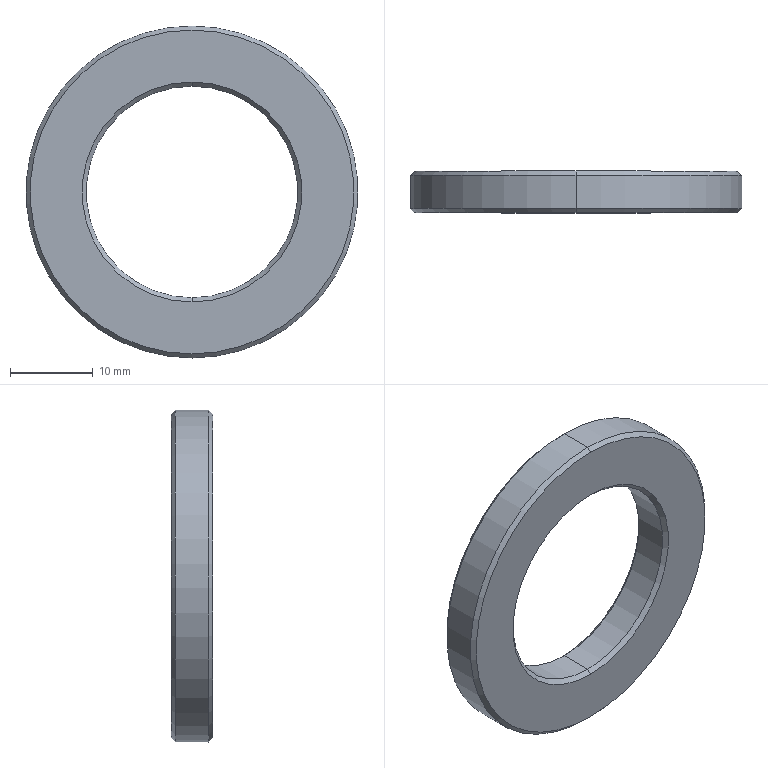Part | SolidWorks | features BaseBody 1 | 1 solid | 14 faces | box 40 x 5 x 40 mm | volume 3678 mm3 | cone 8 | cylinder 4 | plane 2 | commonest cylinder face diameters 25.5 x2 40 x2
STEP:
#1=CARTESIAN_POINT('',(0.,4.5,-12.75));
#2=VERTEX_POINT('',#1);
#3=CARTESIAN_POINT('',(0.,4.5,12.75));
#4=VERTEX_POINT('',#3);
#5=CARTESIAN_POINT('',(0.,4.5,0.));
#6=DIRECTION('',(0.,1.,0.));
#7=DIRECTION('',(0.,0.,-1.));
#8=AXIS2_PLACEMENT_3D('',#5,#6,#7);
#9=CIRCLE('',#8,12.75);
#10=EDGE_CURVE('',#2,#4,#9,.T.);
#11=ORIENTED_EDGE('',*,*,#10,.F.);
#12=CARTESIAN_POINT('',(0.,5.,-13.25));
#13=VERTEX_POINT('',#12);
#14=CARTESIAN_POINT('',(0.,5.,-13.25));
#15=DIRECTION('',(0.,0.7071,-0.7071));
#16=VECTOR('',#15,1000.);
#17=LINE('',#14,#16);
#18=EDGE_CURVE('',#2,#13,#17,.T.);
#19=ORIENTED_EDGE('',*,*,#18,.T.);
#20=CARTESIAN_POINT('',(0.,5.,13.25));
#21=VERTEX_POINT('',#20);
#22=CARTESIAN_POINT('',(0.,5.,0.));
#23=DIRECTION('',(0.,-1.,0.));
#24=DIRECTION('',(0.,0.,1.));
#25=AXIS2_PLACEMENT_3D('',#22,#23,#24);
#26=CIRCLE('',#25,13.25);
#27=EDGE_CURVE('',#21,#13,#26,.T.);
#28=ORIENTED_EDGE('',*,*,#27,.F.);
#29=CARTESIAN_POINT('',(0.,5.,13.25));
#30=DIRECTION('',(0.,0.7071,0.7071));
#31=VECTOR('',#30,1000.);
#32=LINE('',#29,#31);
#33=EDGE_CURVE('',#4,#21,#32,.T.);
#34=ORIENTED_EDGE('',*,*,#33,.F.);
#35=EDGE_LOOP('',(#11,#19,#28,#34));
#36=FACE_OUTER_BOUND('',#35,.T.);
#37=CARTESIAN_POINT('',(0.,5.,0.));
#38=DIRECTION('',(0.,1.,0.));
#39=DIRECTION('',(0.,0.,1.));
#40=AXIS2_PLACEMENT_3D('',#37,#38,#39);
#41=CONICAL_SURFACE('',#40,13.25,0.7854);
#42=ADVANCED_FACE('',(#36),#41,.F.);
#43=CARTESIAN_POINT('',(0.,5.,19.5));
#44=VERTEX_POINT('',#43);
#45=CARTESIAN_POINT('',(0.,5.,-19.5));
#46=VERTEX_POINT('',#45);
#47=CARTESIAN_POINT('',(0.,5.,0.));
#48=DIRECTION('',(0.,1.,0.));
#49=DIRECTION('',(0.,0.,-1.));
#50=AXIS2_PLACEMENT_3D('',#47,#48,#49);
#51=CIRCLE('',#50,19.5);
#52=EDGE_CURVE('',#44,#46,#51,.T.);
#53=ORIENTED_EDGE('',*,*,#52,.F.);
#54=CARTESIAN_POINT('',(0.,4.5,20.));
#55=VERTEX_POINT('',#54);
#56=CARTESIAN_POINT('',(0.,4.5,20.));
#57=DIRECTION('',(0.,-0.7071,0.7071));
#58=VECTOR('',#57,1000.);
#59=LINE('',#56,#58);
#60=EDGE_CURVE('',#44,#55,#59,.T.);
#61=ORIENTED_EDGE('',*,*,#60,.T.);
#62=CARTESIAN_POINT('',(0.,4.5,-20.));
#63=VERTEX_POINT('',#62);
#64=CARTESIAN_POINT('',(0.,4.5,0.));
#65=DIRECTION('',(0.,1.,0.));
#66=DIRECTION('',(0.,0.,-1.));
#67=AXIS2_PLACEMENT_3D('',#64,#65,#66);
#68=CIRCLE('',#67,20.);
#69=EDGE_CURVE('',#55,#63,#68,.T.);
#70=ORIENTED_EDGE('',*,*,#69,.T.);
#71=CARTESIAN_POINT('',(0.,4.5,-20.));
#72=DIRECTION('',(0.,-0.7071,-0.7071));
#73=VECTOR('',#72,1000.);
#74=LINE('',#71,#73);
#75=EDGE_CURVE('',#46,#63,#74,.T.);
#76=ORIENTED_EDGE('',*,*,#75,.F.);
#77=EDGE_LOOP('',(#53,#61,#70,#76));
#78=FACE_OUTER_BOUND('',#77,.T.);
#79=CARTESIAN_POINT('',(0.,4.5,0.));
#80=DIRECTION('',(0.,-1.,0.));
#81=DIRECTION('',(0.,0.,-1.));
#82=AXIS2_PLACEMENT_3D('',#79,#80,#81);
#83=CONICAL_SURFACE('',#82,20.,0.7854);
#84=ADVANCED_FACE('',(#78),#83,.T.);
#85=CARTESIAN_POINT('',(0.,0.5,-12.75));
#86=VERTEX_POINT('',#85);
#87=CARTESIAN_POINT('',(0.,0.5,12.75));
#88=VERTEX_POINT('',#87);
#89=CARTESIAN_POINT('',(0.,0.5,0.));
#90=DIRECTION('',(0.,1.,0.));
#91=DIRECTION('',(0.,0.,1.));
#92=AXIS2_PLACEMENT_3D('',#89,#90,#91);
#93=CIRCLE('',#92,12.75);
#94=EDGE_CURVE('',#86,#88,#93,.T.);
#95=ORIENTED_EDGE('',*,*,#94,.F.);
#96=CARTESIAN_POINT('',(0.,0.,-12.75));
#97=DIRECTION('',(0.,1.,0.));
#98=VECTOR('',#97,1000.);
#99=LINE('',#96,#98);
#100=EDGE_CURVE('',#86,#2,#99,.T.);
#101=ORIENTED_EDGE('',*,*,#100,.T.);
#102=ORIENTED_EDGE('',*,*,#10,.T.);
#103=CARTESIAN_POINT('',(0.,0.,12.75));
#104=DIRECTION('',(0.,1.,0.));
#105=VECTOR('',#104,1000.);
#106=LINE('',#103,#105);
#107=EDGE_CURVE('',#88,#4,#106,.T.);
#108=ORIENTED_EDGE('',*,*,#107,.F.);
#109=EDGE_LOOP('',(#95,#101,#102,#108));
#110=FACE_OUTER_BOUND('',#109,.T.);
#111=CARTESIAN_POINT('',(0.,0.,0.));
#112=DIRECTION('',(0.,1.,0.));
#113=DIRECTION('',(0.,0.,1.));
#114=AXIS2_PLACEMENT_3D('',#111,#112,#113);
#115=CYLINDRICAL_SURFACE('',#114,12.75);
#116=ADVANCED_FACE('',(#110),#115,.F.);
#117=CARTESIAN_POINT('',(0.,0.5,20.));
#118=VERTEX_POINT('',#117);
#119=CARTESIAN_POINT('',(0.,0.5,-20.));
#120=VERTEX_POINT('',#119);
#121=CARTESIAN_POINT('',(0.,0.5,0.));
#122=DIRECTION('',(0.,1.,0.));
#123=DIRECTION('',(0.,0.,1.));
#124=AXIS2_PLACEMENT_3D('',#121,#122,#123);
#125=CIRCLE('',#124,20.);
#126=EDGE_CURVE('',#118,#120,#125,.T.);
#127=ORIENTED_EDGE('',*,*,#126,.T.);
#128=CARTESIAN_POINT('',(0.,0.,-20.));
#129=DIRECTION('',(0.,1.,0.));
#130=VECTOR('',#129,1000.);
#131=LINE('',#128,#130);
#132=EDGE_CURVE('',#120,#63,#131,.T.);
#133=ORIENTED_EDGE('',*,*,#132,.T.);
#134=ORIENTED_EDGE('',*,*,#69,.F.);
#135=CARTESIAN_POINT('',(0.,0.,20.));
#136=DIRECTION('',(0.,1.,0.));
#137=VECTOR('',#136,1000.);
#138=LINE('',#135,#137);
#139=EDGE_CURVE('',#118,#55,#138,.T.);
#140=ORIENTED_EDGE('',*,*,#139,.F.);
#141=EDGE_LOOP('',(#127,#133,#134,#140));
#142=FACE_OUTER_BOUND('',#141,.T.);
#143=CARTESIAN_POINT('',(0.,0.,0.));
#144=DIRECTION('',(0.,1.,0.));
#145=DIRECTION('',(0.,0.,1.));
#146=AXIS2_PLACEMENT_3D('',#143,#144,#145);
#147=CYLINDRICAL_SURFACE('',#146,20.);
#148=ADVANCED_FACE('',(#142),#147,.T.);
#149=ORIENTED_EDGE('',*,*,#94,.T.);
#150=CARTESIAN_POINT('',(0.,0.,13.25));
#151=VERTEX_POINT('',#150);
#152=CARTESIAN_POINT('',(0.,0.,13.25));
#153=DIRECTION('',(0.,-0.7071,0.7071));
#154=VECTOR('',#153,1000.);
#155=LINE('',#152,#154);
#156=EDGE_CURVE('',#88,#151,#155,.T.);
#157=ORIENTED_EDGE('',*,*,#156,.T.);
#158=CARTESIAN_POINT('',(0.,0.,-13.25));
#159=VERTEX_POINT('',#158);
#160=CARTESIAN_POINT('',(0.,0.,0.));
#161=DIRECTION('',(0.,1.,0.));
#162=DIRECTION('',(0.,0.,-1.));
#163=AXIS2_PLACEMENT_3D('',#160,#161,#162);
#164=CIRCLE('',#163,13.25);
#165=EDGE_CURVE('',#159,#151,#164,.T.);
#166=ORIENTED_EDGE('',*,*,#165,.F.);
#167=CARTESIAN_POINT('',(0.,0.,-13.25));
#168=DIRECTION('',(0.,-0.7071,-0.7071));
#169=VECTOR('',#168,1000.);
#170=LINE('',#167,#169);
#171=EDGE_CURVE('',#86,#159,#170,.T.);
#172=ORIENTED_EDGE('',*,*,#171,.F.);
#173=EDGE_LOOP('',(#149,#157,#166,#172));
#174=FACE_OUTER_BOUND('',#173,.T.);
#175=CARTESIAN_POINT('',(0.,0.,0.));
#176=DIRECTION('',(0.,-1.,0.));
#177=DIRECTION('',(0.,0.,-1.));
#178=AXIS2_PLACEMENT_3D('',#175,#176,#177);
#179=CONICAL_SURFACE('',#178,13.25,0.7854);
#180=ADVANCED_FACE('',(#174),#179,.F.);
#181=CARTESIAN_POINT('',(0.,0.,19.5));
#182=VERTEX_POINT('',#181);
#183=CARTESIAN_POINT('',(0.,0.,-19.5));
#184=VERTEX_POINT('',#183);
#185=CARTESIAN_POINT('',(0.,0.,0.));
#186=DIRECTION('',(0.,1.,0.));
#187=DIRECTION('',(0.,0.,1.));
#188=AXIS2_PLACEMENT_3D('',#185,#186,#187);
#189=CIRCLE('',#188,19.5);
#190=EDGE_CURVE('',#182,#184,#189,.T.);
#191=ORIENTED_EDGE('',*,*,#190,.T.);
#192=CARTESIAN_POINT('',(0.,0.5,-20.));
#193=DIRECTION('',(0.,0.7071,-0.7071));
#194=VECTOR('',#193,1000.);
#195=LINE('',#192,#194);
#196=EDGE_CURVE('',#184,#120,#195,.T.);
#197=ORIENTED_EDGE('',*,*,#196,.T.);
#198=ORIENTED_EDGE('',*,*,#126,.F.);
#199=CARTESIAN_POINT('',(0.,0.5,20.));
#200=DIRECTION('',(0.,0.7071,0.7071));
#201=VECTOR('',#200,1000.);
#202=LINE('',#199,#201);
#203=EDGE_CURVE('',#182,#118,#202,.T.);
#204=ORIENTED_EDGE('',*,*,#203,.F.);
#205=EDGE_LOOP('',(#191,#197,#198,#204));
#206=FACE_OUTER_BOUND('',#205,.T.);
#207=CARTESIAN_POINT('',(0.,0.5,0.));
#208=DIRECTION('',(0.,1.,0.));
#209=DIRECTION('',(0.,0.,1.));
#210=AXIS2_PLACEMENT_3D('',#207,#208,#209);
#211=CONICAL_SURFACE('',#210,20.,0.7854);
#212=ADVANCED_FACE('',(#206),#211,.T.);
#213=ORIENTED_EDGE('',*,*,#27,.T.);
#214=CARTESIAN_POINT('',(0.,5.,0.));
#215=DIRECTION('',(0.,-1.,0.));
#216=DIRECTION('',(0.,0.,1.));
#217=AXIS2_PLACEMENT_3D('',#214,#215,#216);
#218=CIRCLE('',#217,13.25);
#219=EDGE_CURVE('',#13,#21,#218,.T.);
#220=ORIENTED_EDGE('',*,*,#219,.T.);
#221=EDGE_LOOP('',(#213,#220));
#222=FACE_BOUND('',#221,.T.);
#223=CARTESIAN_POINT('',(0.,5.,0.));
#224=DIRECTION('',(0.,1.,0.));
#225=DIRECTION('',(0.,0.,-1.));
#226=AXIS2_PLACEMENT_3D('',#223,#224,#225);
#227=CIRCLE('',#226,19.5);
#228=EDGE_CURVE('',#46,#44,#227,.T.);
#229=ORIENTED_EDGE('',*,*,#228,.T.);
#230=ORIENTED_EDGE('',*,*,#52,.T.);
#231=EDGE_LOOP('',(#229,#230));
#232=FACE_OUTER_BOUND('',#231,.T.);
#233=CARTESIAN_POINT('',(0.,5.,0.));
#234=DIRECTION('',(0.,1.,0.));
#235=DIRECTION('',(0.,0.,1.));
#236=AXIS2_PLACEMENT_3D('',#233,#234,#235);
#237=PLANE('',#236);
#238=ADVANCED_FACE('',(#222,#232),#237,.T.);
#239=ORIENTED_EDGE('',*,*,#18,.F.);
#240=CARTESIAN_POINT('',(0.,4.5,0.));
#241=DIRECTION('',(0.,1.,0.));
#242=DIRECTION('',(0.,0.,-1.));
#243=AXIS2_PLACEMENT_3D('',#240,#241,#242);
#244=CIRCLE('',#243,12.75);
#245=EDGE_CURVE('',#4,#2,#244,.T.);
#246=ORIENTED_EDGE('',*,*,#245,.F.);
#247=ORIENTED_EDGE('',*,*,#33,.T.);
#248=ORIENTED_EDGE('',*,*,#219,.F.);
#249=EDGE_LOOP('',(#239,#246,#247,#248));
#250=FACE_OUTER_BOUND('',#249,.T.);
#251=CARTESIAN_POINT('',(0.,5.,0.));
#252=DIRECTION('',(0.,1.,0.));
#253=DIRECTION('',(0.,0.,1.));
#254=AXIS2_PLACEMENT_3D('',#251,#252,#253);
#255=CONICAL_SURFACE('',#254,13.25,0.7854);
#256=ADVANCED_FACE('',(#250),#255,.F.);
#257=ORIENTED_EDGE('',*,*,#60,.F.);
#258=ORIENTED_EDGE('',*,*,#228,.F.);
#259=ORIENTED_EDGE('',*,*,#75,.T.);
#260=CARTESIAN_POINT('',(0.,4.5,0.));
#261=DIRECTION('',(0.,1.,0.));
#262=DIRECTION('',(0.,0.,-1.));
#263=AXIS2_PLACEMENT_3D('',#260,#261,#262);
#264=CIRCLE('',#263,20.);
#265=EDGE_CURVE('',#63,#55,#264,.T.);
#266=ORIENTED_EDGE('',*,*,#265,.T.);
#267=EDGE_LOOP('',(#257,#258,#259,#266));
#268=FACE_OUTER_BOUND('',#267,.T.);
#269=CARTESIAN_POINT('',(0.,4.5,0.));
#270=DIRECTION('',(0.,-1.,0.));
#271=DIRECTION('',(0.,0.,-1.));
#272=AXIS2_PLACEMENT_3D('',#269,#270,#271);
#273=CONICAL_SURFACE('',#272,20.,0.7854);
#274=ADVANCED_FACE('',(#268),#273,.T.);
#275=ORIENTED_EDGE('',*,*,#100,.F.);
#276=CARTESIAN_POINT('',(0.,0.5,0.));
#277=DIRECTION('',(0.,1.,0.));
#278=DIRECTION('',(0.,0.,1.));
#279=AXIS2_PLACEMENT_3D('',#276,#277,#278);
#280=CIRCLE('',#279,12.75);
#281=EDGE_CURVE('',#88,#86,#280,.T.);
#282=ORIENTED_EDGE('',*,*,#281,.F.);
#283=ORIENTED_EDGE('',*,*,#107,.T.);
#284=ORIENTED_EDGE('',*,*,#245,.T.);
#285=EDGE_LOOP('',(#275,#282,#283,#284));
#286=FACE_OUTER_BOUND('',#285,.T.);
#287=CARTESIAN_POINT('',(0.,0.,0.));
#288=DIRECTION('',(0.,1.,0.));
#289=DIRECTION('',(0.,0.,1.));
#290=AXIS2_PLACEMENT_3D('',#287,#288,#289);
#291=CYLINDRICAL_SURFACE('',#290,12.75);
#292=ADVANCED_FACE('',(#286),#291,.F.);
#293=ORIENTED_EDGE('',*,*,#132,.F.);
#294=CARTESIAN_POINT('',(0.,0.5,0.));
#295=DIRECTION('',(0.,1.,0.));
#296=DIRECTION('',(0.,0.,1.));
#297=AXIS2_PLACEMENT_3D('',#294,#295,#296);
#298=CIRCLE('',#297,20.);
#299=EDGE_CURVE('',#120,#118,#298,.T.);
#300=ORIENTED_EDGE('',*,*,#299,.T.);
#301=ORIENTED_EDGE('',*,*,#139,.T.);
#302=ORIENTED_EDGE('',*,*,#265,.F.);
#303=EDGE_LOOP('',(#293,#300,#301,#302));
#304=FACE_OUTER_BOUND('',#303,.T.);
#305=CARTESIAN_POINT('',(0.,0.,0.));
#306=DIRECTION('',(0.,1.,0.));
#307=DIRECTION('',(0.,0.,1.));
#308=AXIS2_PLACEMENT_3D('',#305,#306,#307);
#309=CYLINDRICAL_SURFACE('',#308,20.);
#310=ADVANCED_FACE('',(#304),#309,.T.);
#311=ORIENTED_EDGE('',*,*,#156,.F.);
#312=ORIENTED_EDGE('',*,*,#281,.T.);
#313=ORIENTED_EDGE('',*,*,#171,.T.);
#314=CARTESIAN_POINT('',(0.,0.,0.));
#315=DIRECTION('',(0.,1.,0.));
#316=DIRECTION('',(0.,0.,-1.));
#317=AXIS2_PLACEMENT_3D('',#314,#315,#316);
#318=CIRCLE('',#317,13.25);
#319=EDGE_CURVE('',#151,#159,#318,.T.);
#320=ORIENTED_EDGE('',*,*,#319,.F.);
#321=EDGE_LOOP('',(#311,#312,#313,#320));
#322=FACE_OUTER_BOUND('',#321,.T.);
#323=CARTESIAN_POINT('',(0.,0.,0.));
#324=DIRECTION('',(0.,-1.,0.));
#325=DIRECTION('',(0.,0.,-1.));
#326=AXIS2_PLACEMENT_3D('',#323,#324,#325);
#327=CONICAL_SURFACE('',#326,13.25,0.7854);
#328=ADVANCED_FACE('',(#322),#327,.F.);
#329=ORIENTED_EDGE('',*,*,#196,.F.);
#330=CARTESIAN_POINT('',(0.,0.,0.));
#331=DIRECTION('',(0.,1.,0.));
#332=DIRECTION('',(0.,0.,1.));
#333=AXIS2_PLACEMENT_3D('',#330,#331,#332);
#334=CIRCLE('',#333,19.5);
#335=EDGE_CURVE('',#184,#182,#334,.T.);
#336=ORIENTED_EDGE('',*,*,#335,.T.);
#337=ORIENTED_EDGE('',*,*,#203,.T.);
#338=ORIENTED_EDGE('',*,*,#299,.F.);
#339=EDGE_LOOP('',(#329,#336,#337,#338));
#340=FACE_OUTER_BOUND('',#339,.T.);
#341=CARTESIAN_POINT('',(0.,0.5,0.));
#342=DIRECTION('',(0.,1.,0.));
#343=DIRECTION('',(0.,0.,1.));
#344=AXIS2_PLACEMENT_3D('',#341,#342,#343);
#345=CONICAL_SURFACE('',#344,20.,0.7854);
#346=ADVANCED_FACE('',(#340),#345,.T.);
#347=ORIENTED_EDGE('',*,*,#165,.T.);
#348=ORIENTED_EDGE('',*,*,#319,.T.);
#349=EDGE_LOOP('',(#347,#348));
#350=FACE_BOUND('',#349,.T.);
#351=ORIENTED_EDGE('',*,*,#190,.F.);
#352=ORIENTED_EDGE('',*,*,#335,.F.);
#353=EDGE_LOOP('',(#351,#352));
#354=FACE_OUTER_BOUND('',#353,.T.);
#355=CARTESIAN_POINT('',(0.,0.,0.));
#356=DIRECTION('',(0.,1.,0.));
#357=DIRECTION('',(0.,0.,1.));
#358=AXIS2_PLACEMENT_3D('',#355,#356,#357);
#359=PLANE('',#358);
#360=ADVANCED_FACE('',(#350,#354),#359,.F.);
#361=CLOSED_SHELL('',(#42,#84,#116,#148,#180,#212,#238,#256,#274,#292,#310,#328,#346,#360));
#362=MANIFOLD_SOLID_BREP('',#361);
#363=CARTESIAN_POINT('',(0.,0.,0.));
#364=DIRECTION('',(0.,0.,1.));
#365=DIRECTION('',(1.,0.,0.));
#366=AXIS2_PLACEMENT_3D('',#363,#364,#365);
#367=(LENGTH_UNIT()NAMED_UNIT(*)SI_UNIT(.MILLI.,.METRE.));
#368=UNCERTAINTY_MEASURE_WITH_UNIT(LENGTH_MEASURE(0.00001),#367,'','');
#369=(NAMED_UNIT(*)PLANE_ANGLE_UNIT()SI_UNIT($,.RADIAN.));
#370=(NAMED_UNIT(*)SI_UNIT($,.STERADIAN.)SOLID_ANGLE_UNIT());
#371=(GEOMETRIC_REPRESENTATION_CONTEXT(3)GLOBAL_UNCERTAINTY_ASSIGNED_CONTEXT((#368))GLOBAL_UNIT_ASSIGNED_CONTEXT((#367,#369,#370))REPRESENTATION_CONTEXT('',''));
#372=ADVANCED_BREP_SHAPE_REPRESENTATION('',(#362,#366),#371);